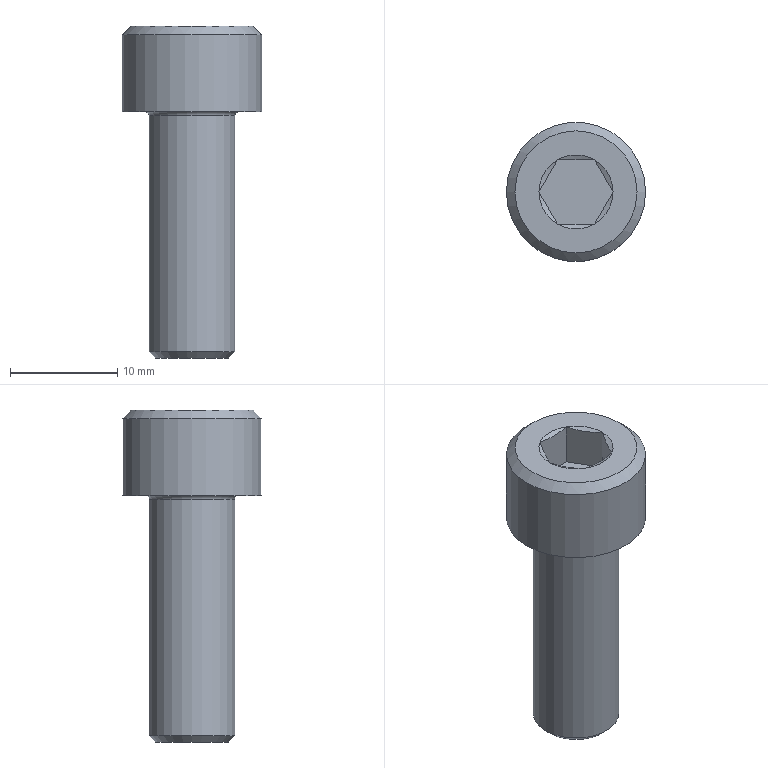Part | STEP file | solid 19 | 1 solid | 21 faces | box 13 x 13 x 31 mm | volume 2077 mm3 | plane 10 | sphere 6 | cylinder 2 | cone 2 | torus 1 | commonest cylinder face diameters 8 x1 13 x1